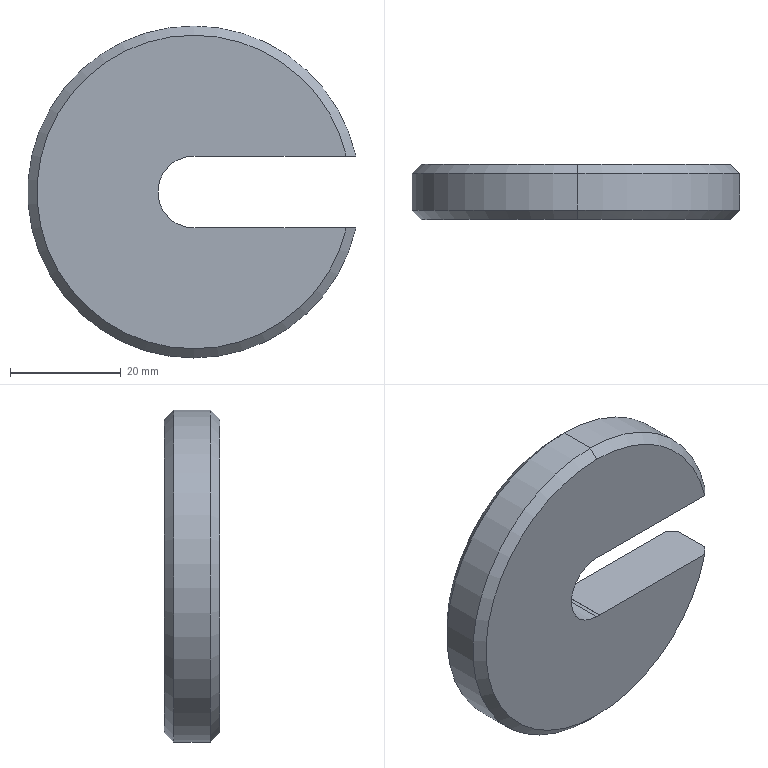Part | SolidWorks | features ICE 2, Chamfer 1, Extrusion 1 | 1 solid | 18 faces | box 59.287 x 10 x 60 mm | volume 23262 mm3 | cone 6 | cylinder 6 | plane 6 | commonest cylinder face diameters 13 x3 60 x3
STEP:
#1=CARTESIAN_POINT('',(0.,10.,28.33));
#2=VERTEX_POINT('',#1);
#3=CARTESIAN_POINT('',(27.574,10.,6.5));
#4=VERTEX_POINT('',#3);
#5=CARTESIAN_POINT('',(0.,10.,0.));
#6=DIRECTION('',(0.,1.,0.));
#7=DIRECTION('',(0.,0.,1.));
#8=AXIS2_PLACEMENT_3D('',#5,#6,#7);
#9=CIRCLE('',#8,28.33);
#10=EDGE_CURVE('',#2,#4,#9,.T.);
#11=ORIENTED_EDGE('',*,*,#10,.F.);
#12=CARTESIAN_POINT('',(0.,8.33,30.));
#13=VERTEX_POINT('',#12);
#14=CARTESIAN_POINT('',(0.,10.,28.33));
#15=DIRECTION('',(0.,-0.7071,0.7071));
#16=VECTOR('',#15,1000.);
#17=LINE('',#14,#16);
#18=EDGE_CURVE('',#2,#13,#17,.T.);
#19=ORIENTED_EDGE('',*,*,#18,.T.);
#20=CARTESIAN_POINT('',(29.287,8.33,6.5));
#21=VERTEX_POINT('',#20);
#22=CARTESIAN_POINT('',(0.,8.33,0.));
#23=DIRECTION('',(0.,-1.,0.));
#24=DIRECTION('',(0.,0.,1.));
#25=AXIS2_PLACEMENT_3D('',#22,#23,#24);
#26=CIRCLE('',#25,30.);
#27=EDGE_CURVE('',#21,#13,#26,.T.);
#28=ORIENTED_EDGE('',*,*,#27,.F.);
#29=CARTESIAN_POINT('',(27.574,10.,6.5));
#30=CARTESIAN_POINT('',(28.146,9.444,6.5));
#31=CARTESIAN_POINT('',(28.717,8.887,6.5));
#32=CARTESIAN_POINT('',(29.287,8.33,6.5));
#33=B_SPLINE_CURVE_WITH_KNOTS('',3,(#29,#30,#31,#32),.UNSPECIFIED.,.F.,.F.,(4,4),(0.,0.002392),.UNSPECIFIED.);
#34=EDGE_CURVE('',#4,#21,#33,.T.);
#35=ORIENTED_EDGE('',*,*,#34,.F.);
#36=EDGE_LOOP('',(#11,#19,#28,#35));
#37=FACE_OUTER_BOUND('',#36,.T.);
#38=CARTESIAN_POINT('',(0.,10.,0.));
#39=DIRECTION('',(0.,-1.,0.));
#40=DIRECTION('',(0.,0.,-1.));
#41=AXIS2_PLACEMENT_3D('',#38,#39,#40);
#42=CONICAL_SURFACE('',#41,28.33,0.7854);
#43=ADVANCED_FACE('',(#37),#42,.T.);
#44=ORIENTED_EDGE('',*,*,#18,.F.);
#45=CARTESIAN_POINT('',(0.,10.,-28.33));
#46=VERTEX_POINT('',#45);
#47=CARTESIAN_POINT('',(0.,10.,0.));
#48=DIRECTION('',(0.,1.,0.));
#49=DIRECTION('',(0.,0.,1.));
#50=AXIS2_PLACEMENT_3D('',#47,#48,#49);
#51=CIRCLE('',#50,28.33);
#52=EDGE_CURVE('',#46,#2,#51,.T.);
#53=ORIENTED_EDGE('',*,*,#52,.F.);
#54=CARTESIAN_POINT('',(0.,8.33,-30.));
#55=VERTEX_POINT('',#54);
#56=CARTESIAN_POINT('',(0.,10.,-28.33));
#57=DIRECTION('',(0.,-0.7071,-0.7071));
#58=VECTOR('',#57,1000.);
#59=LINE('',#56,#58);
#60=EDGE_CURVE('',#46,#55,#59,.T.);
#61=ORIENTED_EDGE('',*,*,#60,.T.);
#62=CARTESIAN_POINT('',(0.,8.33,0.));
#63=DIRECTION('',(0.,-1.,0.));
#64=DIRECTION('',(0.,0.,1.));
#65=AXIS2_PLACEMENT_3D('',#62,#63,#64);
#66=CIRCLE('',#65,30.);
#67=EDGE_CURVE('',#13,#55,#66,.T.);
#68=ORIENTED_EDGE('',*,*,#67,.F.);
#69=EDGE_LOOP('',(#44,#53,#61,#68));
#70=FACE_OUTER_BOUND('',#69,.T.);
#71=CARTESIAN_POINT('',(0.,10.,0.));
#72=DIRECTION('',(0.,-1.,0.));
#73=DIRECTION('',(0.,0.,-1.));
#74=AXIS2_PLACEMENT_3D('',#71,#72,#73);
#75=CONICAL_SURFACE('',#74,28.33,0.7854);
#76=ADVANCED_FACE('',(#70),#75,.T.);
#77=CARTESIAN_POINT('',(0.,0.,-28.33));
#78=VERTEX_POINT('',#77);
#79=CARTESIAN_POINT('',(27.574,0.,-6.5));
#80=VERTEX_POINT('',#79);
#81=CARTESIAN_POINT('',(0.,0.,0.));
#82=DIRECTION('',(0.,-1.,0.));
#83=DIRECTION('',(0.,0.,1.));
#84=AXIS2_PLACEMENT_3D('',#81,#82,#83);
#85=CIRCLE('',#84,28.33);
#86=EDGE_CURVE('',#78,#80,#85,.T.);
#87=ORIENTED_EDGE('',*,*,#86,.F.);
#88=CARTESIAN_POINT('',(0.,1.67,-30.));
#89=VERTEX_POINT('',#88);
#90=CARTESIAN_POINT('',(0.,1.67,-30.));
#91=DIRECTION('',(0.,0.7071,-0.7071));
#92=VECTOR('',#91,1000.);
#93=LINE('',#90,#92);
#94=EDGE_CURVE('',#78,#89,#93,.T.);
#95=ORIENTED_EDGE('',*,*,#94,.T.);
#96=CARTESIAN_POINT('',(29.287,1.67,-6.5));
#97=VERTEX_POINT('',#96);
#98=CARTESIAN_POINT('',(0.,1.67,0.));
#99=DIRECTION('',(0.,1.,0.));
#100=DIRECTION('',(0.,0.,1.));
#101=AXIS2_PLACEMENT_3D('',#98,#99,#100);
#102=CIRCLE('',#101,30.);
#103=EDGE_CURVE('',#97,#89,#102,.T.);
#104=ORIENTED_EDGE('',*,*,#103,.F.);
#105=CARTESIAN_POINT('',(27.574,0.,-6.5));
#106=CARTESIAN_POINT('',(28.146,0.5562,-6.5));
#107=CARTESIAN_POINT('',(28.717,1.113,-6.5));
#108=CARTESIAN_POINT('',(29.287,1.67,-6.5));
#109=B_SPLINE_CURVE_WITH_KNOTS('',3,(#105,#106,#107,#108),.UNSPECIFIED.,.F.,.F.,(4,4),(0.,0.002392),.UNSPECIFIED.);
#110=EDGE_CURVE('',#80,#97,#109,.T.);
#111=ORIENTED_EDGE('',*,*,#110,.F.);
#112=EDGE_LOOP('',(#87,#95,#104,#111));
#113=FACE_OUTER_BOUND('',#112,.T.);
#114=CARTESIAN_POINT('',(0.,1.67,0.));
#115=DIRECTION('',(0.,1.,0.));
#116=DIRECTION('',(0.,0.,1.));
#117=AXIS2_PLACEMENT_3D('',#114,#115,#116);
#118=CONICAL_SURFACE('',#117,30.,0.7854);
#119=ADVANCED_FACE('',(#113),#118,.T.);
#120=ORIENTED_EDGE('',*,*,#94,.F.);
#121=CARTESIAN_POINT('',(0.,0.,28.33));
#122=VERTEX_POINT('',#121);
#123=CARTESIAN_POINT('',(0.,0.,0.));
#124=DIRECTION('',(0.,-1.,0.));
#125=DIRECTION('',(0.,0.,1.));
#126=AXIS2_PLACEMENT_3D('',#123,#124,#125);
#127=CIRCLE('',#126,28.33);
#128=EDGE_CURVE('',#122,#78,#127,.T.);
#129=ORIENTED_EDGE('',*,*,#128,.F.);
#130=CARTESIAN_POINT('',(0.,1.67,30.));
#131=VERTEX_POINT('',#130);
#132=CARTESIAN_POINT('',(0.,1.67,30.));
#133=DIRECTION('',(0.,0.7071,0.7071));
#134=VECTOR('',#133,1000.);
#135=LINE('',#132,#134);
#136=EDGE_CURVE('',#122,#131,#135,.T.);
#137=ORIENTED_EDGE('',*,*,#136,.T.);
#138=CARTESIAN_POINT('',(0.,1.67,0.));
#139=DIRECTION('',(0.,1.,0.));
#140=DIRECTION('',(0.,0.,1.));
#141=AXIS2_PLACEMENT_3D('',#138,#139,#140);
#142=CIRCLE('',#141,30.);
#143=EDGE_CURVE('',#89,#131,#142,.T.);
#144=ORIENTED_EDGE('',*,*,#143,.F.);
#145=EDGE_LOOP('',(#120,#129,#137,#144));
#146=FACE_OUTER_BOUND('',#145,.T.);
#147=CARTESIAN_POINT('',(0.,1.67,0.));
#148=DIRECTION('',(0.,1.,0.));
#149=DIRECTION('',(0.,0.,1.));
#150=AXIS2_PLACEMENT_3D('',#147,#148,#149);
#151=CONICAL_SURFACE('',#150,30.,0.7854);
#152=ADVANCED_FACE('',(#146),#151,.T.);
#153=CARTESIAN_POINT('',(0.,0.,-6.5));
#154=VERTEX_POINT('',#153);
#155=CARTESIAN_POINT('',(0.,0.,6.5));
#156=VERTEX_POINT('',#155);
#157=CARTESIAN_POINT('',(0.,0.,0.));
#158=DIRECTION('',(0.,1.,0.));
#159=DIRECTION('',(0.,0.,1.));
#160=AXIS2_PLACEMENT_3D('',#157,#158,#159);
#161=CIRCLE('',#160,6.5);
#162=EDGE_CURVE('',#154,#156,#161,.T.);
#163=ORIENTED_EDGE('',*,*,#162,.F.);
#164=CARTESIAN_POINT('',(0.,10.,-6.5));
#165=VERTEX_POINT('',#164);
#166=CARTESIAN_POINT('',(0.,-23.,-6.5));
#167=DIRECTION('',(0.,1.,0.));
#168=VECTOR('',#167,1000.);
#169=LINE('',#166,#168);
#170=EDGE_CURVE('',#154,#165,#169,.T.);
#171=ORIENTED_EDGE('',*,*,#170,.T.);
#172=CARTESIAN_POINT('',(0.,10.,6.5));
#173=VERTEX_POINT('',#172);
#174=CARTESIAN_POINT('',(0.,10.,0.));
#175=DIRECTION('',(0.,1.,0.));
#176=DIRECTION('',(0.,0.,1.));
#177=AXIS2_PLACEMENT_3D('',#174,#175,#176);
#178=CIRCLE('',#177,6.5);
#179=EDGE_CURVE('',#165,#173,#178,.T.);
#180=ORIENTED_EDGE('',*,*,#179,.T.);
#181=CARTESIAN_POINT('',(0.,-23.,6.5));
#182=DIRECTION('',(0.,1.,0.));
#183=VECTOR('',#182,1000.);
#184=LINE('',#181,#183);
#185=EDGE_CURVE('',#156,#173,#184,.T.);
#186=ORIENTED_EDGE('',*,*,#185,.F.);
#187=EDGE_LOOP('',(#163,#171,#180,#186));
#188=FACE_OUTER_BOUND('',#187,.T.);
#189=CARTESIAN_POINT('',(0.,-23.,0.));
#190=DIRECTION('',(0.,1.,0.));
#191=DIRECTION('',(0.,0.,1.));
#192=AXIS2_PLACEMENT_3D('',#189,#190,#191);
#193=CYLINDRICAL_SURFACE('',#192,6.5);
#194=ADVANCED_FACE('',(#188),#193,.F.);
#195=CARTESIAN_POINT('',(0.689,0.,6.463));
#196=VERTEX_POINT('',#195);
#197=CARTESIAN_POINT('',(0.,0.,0.));
#198=DIRECTION('',(0.,1.,0.));
#199=DIRECTION('',(0.,0.,1.));
#200=AXIS2_PLACEMENT_3D('',#197,#198,#199);
#201=CIRCLE('',#200,6.5);
#202=EDGE_CURVE('',#156,#196,#201,.T.);
#203=ORIENTED_EDGE('',*,*,#202,.F.);
#204=ORIENTED_EDGE('',*,*,#185,.T.);
#205=CARTESIAN_POINT('',(0.689,10.,6.463));
#206=VERTEX_POINT('',#205);
#207=CARTESIAN_POINT('',(0.,10.,0.));
#208=DIRECTION('',(0.,1.,0.));
#209=DIRECTION('',(0.,0.,1.));
#210=AXIS2_PLACEMENT_3D('',#207,#208,#209);
#211=CIRCLE('',#210,6.5);
#212=EDGE_CURVE('',#173,#206,#211,.T.);
#213=ORIENTED_EDGE('',*,*,#212,.T.);
#214=CARTESIAN_POINT('',(0.689,-23.,6.463));
#215=DIRECTION('',(0.,1.,0.));
#216=VECTOR('',#215,1000.);
#217=LINE('',#214,#216);
#218=EDGE_CURVE('',#196,#206,#217,.T.);
#219=ORIENTED_EDGE('',*,*,#218,.F.);
#220=EDGE_LOOP('',(#203,#204,#213,#219));
#221=FACE_OUTER_BOUND('',#220,.T.);
#222=CARTESIAN_POINT('',(0.,-23.,0.));
#223=DIRECTION('',(0.,1.,0.));
#224=DIRECTION('',(0.,0.,1.));
#225=AXIS2_PLACEMENT_3D('',#222,#223,#224);
#226=CYLINDRICAL_SURFACE('',#225,6.5);
#227=ADVANCED_FACE('',(#221),#226,.F.);
#228=ORIENTED_EDGE('',*,*,#27,.T.);
#229=CARTESIAN_POINT('',(0.,10.,30.));
#230=DIRECTION('',(0.,-1.,0.));
#231=VECTOR('',#230,1000.);
#232=LINE('',#229,#231);
#233=EDGE_CURVE('',#13,#131,#232,.T.);
#234=ORIENTED_EDGE('',*,*,#233,.T.);
#235=CARTESIAN_POINT('',(29.287,1.67,6.5));
#236=VERTEX_POINT('',#235);
#237=CARTESIAN_POINT('',(0.,1.67,0.));
#238=DIRECTION('',(0.,1.,0.));
#239=DIRECTION('',(0.,0.,1.));
#240=AXIS2_PLACEMENT_3D('',#237,#238,#239);
#241=CIRCLE('',#240,30.);
#242=EDGE_CURVE('',#131,#236,#241,.T.);
#243=ORIENTED_EDGE('',*,*,#242,.T.);
#244=CARTESIAN_POINT('',(29.287,10.,6.5));
#245=DIRECTION('',(0.,1.,0.));
#246=VECTOR('',#245,1000.);
#247=LINE('',#244,#246);
#248=EDGE_CURVE('',#236,#21,#247,.T.);
#249=ORIENTED_EDGE('',*,*,#248,.T.);
#250=EDGE_LOOP('',(#228,#234,#243,#249));
#251=FACE_OUTER_BOUND('',#250,.T.);
#252=CARTESIAN_POINT('',(0.,10.,0.));
#253=DIRECTION('',(0.,-1.,0.));
#254=DIRECTION('',(0.,0.,-1.));
#255=AXIS2_PLACEMENT_3D('',#252,#253,#254);
#256=CYLINDRICAL_SURFACE('',#255,30.);
#257=ADVANCED_FACE('',(#251),#256,.T.);
#258=ORIENTED_EDGE('',*,*,#233,.F.);
#259=ORIENTED_EDGE('',*,*,#67,.T.);
#260=CARTESIAN_POINT('',(0.,10.,-30.));
#261=DIRECTION('',(0.,-1.,0.));
#262=VECTOR('',#261,1000.);
#263=LINE('',#260,#262);
#264=EDGE_CURVE('',#55,#89,#263,.T.);
#265=ORIENTED_EDGE('',*,*,#264,.T.);
#266=ORIENTED_EDGE('',*,*,#143,.T.);
#267=EDGE_LOOP('',(#258,#259,#265,#266));
#268=FACE_OUTER_BOUND('',#267,.T.);
#269=CARTESIAN_POINT('',(0.,10.,0.));
#270=DIRECTION('',(0.,-1.,0.));
#271=DIRECTION('',(0.,0.,-1.));
#272=AXIS2_PLACEMENT_3D('',#269,#270,#271);
#273=CYLINDRICAL_SURFACE('',#272,30.);
#274=ADVANCED_FACE('',(#268),#273,.T.);
#275=CARTESIAN_POINT('',(0.689,0.,6.5));
#276=VERTEX_POINT('',#275);
#277=CARTESIAN_POINT('',(0.689,0.,0.));
#278=DIRECTION('',(0.,0.,1.));
#279=VECTOR('',#278,1000.);
#280=LINE('',#277,#279);
#281=EDGE_CURVE('',#196,#276,#280,.T.);
#282=ORIENTED_EDGE('',*,*,#281,.F.);
#283=ORIENTED_EDGE('',*,*,#218,.T.);
#284=CARTESIAN_POINT('',(0.689,10.,6.5));
#285=VERTEX_POINT('',#284);
#286=CARTESIAN_POINT('',(0.689,10.,-6.5));
#287=DIRECTION('',(0.,0.,1.));
#288=VECTOR('',#287,1000.);
#289=LINE('',#286,#288);
#290=EDGE_CURVE('',#206,#285,#289,.T.);
#291=ORIENTED_EDGE('',*,*,#290,.T.);
#292=CARTESIAN_POINT('',(0.689,-23.,6.5));
#293=DIRECTION('',(0.,1.,0.));
#294=VECTOR('',#293,1000.);
#295=LINE('',#292,#294);
#296=EDGE_CURVE('',#276,#285,#295,.T.);
#297=ORIENTED_EDGE('',*,*,#296,.F.);
#298=EDGE_LOOP('',(#282,#283,#291,#297));
#299=FACE_OUTER_BOUND('',#298,.T.);
#300=CARTESIAN_POINT('',(0.689,-23.,-6.5));
#301=DIRECTION('',(-1.,0.,0.));
#302=DIRECTION('',(0.,0.,1.));
#303=AXIS2_PLACEMENT_3D('',#300,#301,#302);
#304=PLANE('',#303);
#305=ADVANCED_FACE('',(#299),#304,.F.);
#306=ORIENTED_EDGE('',*,*,#264,.F.);
#307=CARTESIAN_POINT('',(29.287,8.33,-6.5));
#308=VERTEX_POINT('',#307);
#309=CARTESIAN_POINT('',(0.,8.33,0.));
#310=DIRECTION('',(0.,-1.,0.));
#311=DIRECTION('',(0.,0.,1.));
#312=AXIS2_PLACEMENT_3D('',#309,#310,#311);
#313=CIRCLE('',#312,30.);
#314=EDGE_CURVE('',#55,#308,#313,.T.);
#315=ORIENTED_EDGE('',*,*,#314,.T.);
#316=CARTESIAN_POINT('',(29.287,10.,-6.5));
#317=DIRECTION('',(0.,-1.,0.));
#318=VECTOR('',#317,1000.);
#319=LINE('',#316,#318);
#320=EDGE_CURVE('',#308,#97,#319,.T.);
#321=ORIENTED_EDGE('',*,*,#320,.T.);
#322=ORIENTED_EDGE('',*,*,#103,.T.);
#323=EDGE_LOOP('',(#306,#315,#321,#322));
#324=FACE_OUTER_BOUND('',#323,.T.);
#325=CARTESIAN_POINT('',(0.,10.,0.));
#326=DIRECTION('',(0.,-1.,0.));
#327=DIRECTION('',(0.,0.,-1.));
#328=AXIS2_PLACEMENT_3D('',#325,#326,#327);
#329=CYLINDRICAL_SURFACE('',#328,30.);
#330=ADVANCED_FACE('',(#324),#329,.T.);
#331=CARTESIAN_POINT('',(27.574,10.,-6.5));
#332=VERTEX_POINT('',#331);
#333=CARTESIAN_POINT('',(0.689,10.,-6.5));
#334=VERTEX_POINT('',#333);
#335=CARTESIAN_POINT('',(0.689,10.,-6.5));
#336=DIRECTION('',(-1.,0.,0.));
#337=VECTOR('',#336,1000.);
#338=LINE('',#335,#337);
#339=EDGE_CURVE('',#332,#334,#338,.T.);
#340=ORIENTED_EDGE('',*,*,#339,.F.);
#341=CARTESIAN_POINT('',(0.,10.,0.));
#342=DIRECTION('',(0.,1.,0.));
#343=DIRECTION('',(0.,0.,1.));
#344=AXIS2_PLACEMENT_3D('',#341,#342,#343);
#345=CIRCLE('',#344,28.33);
#346=EDGE_CURVE('',#332,#46,#345,.T.);
#347=ORIENTED_EDGE('',*,*,#346,.T.);
#348=ORIENTED_EDGE('',*,*,#52,.T.);
#349=ORIENTED_EDGE('',*,*,#10,.T.);
#350=CARTESIAN_POINT('',(0.689,10.,6.5));
#351=DIRECTION('',(1.,0.,0.));
#352=VECTOR('',#351,1000.);
#353=LINE('',#350,#352);
#354=EDGE_CURVE('',#285,#4,#353,.T.);
#355=ORIENTED_EDGE('',*,*,#354,.F.);
#356=ORIENTED_EDGE('',*,*,#290,.F.);
#357=ORIENTED_EDGE('',*,*,#212,.F.);
#358=ORIENTED_EDGE('',*,*,#179,.F.);
#359=CARTESIAN_POINT('',(0.689,10.,-6.463));
#360=VERTEX_POINT('',#359);
#361=CARTESIAN_POINT('',(0.,10.,0.));
#362=DIRECTION('',(0.,1.,0.));
#363=DIRECTION('',(0.,0.,1.));
#364=AXIS2_PLACEMENT_3D('',#361,#362,#363);
#365=CIRCLE('',#364,6.5);
#366=EDGE_CURVE('',#360,#165,#365,.T.);
#367=ORIENTED_EDGE('',*,*,#366,.F.);
#368=CARTESIAN_POINT('',(0.689,10.,-6.5));
#369=DIRECTION('',(0.,0.,1.));
#370=VECTOR('',#369,1000.);
#371=LINE('',#368,#370);
#372=EDGE_CURVE('',#334,#360,#371,.T.);
#373=ORIENTED_EDGE('',*,*,#372,.F.);
#374=EDGE_LOOP('',(#340,#347,#348,#349,#355,#356,#357,#358,#367,#373));
#375=FACE_OUTER_BOUND('',#374,.T.);
#376=CARTESIAN_POINT('',(0.,10.,0.));
#377=DIRECTION('',(0.,1.,0.));
#378=DIRECTION('',(0.,0.,1.));
#379=AXIS2_PLACEMENT_3D('',#376,#377,#378);
#380=PLANE('',#379);
#381=ADVANCED_FACE('',(#375),#380,.T.);
#382=CARTESIAN_POINT('',(27.574,0.,6.5));
#383=VERTEX_POINT('',#382);
#384=CARTESIAN_POINT('',(0.,0.,6.5));
#385=DIRECTION('',(1.,0.,0.));
#386=VECTOR('',#385,1000.);
#387=LINE('',#384,#386);
#388=EDGE_CURVE('',#276,#383,#387,.T.);
#389=ORIENTED_EDGE('',*,*,#388,.T.);
#390=CARTESIAN_POINT('',(0.,0.,0.));
#391=DIRECTION('',(0.,-1.,0.));
#392=DIRECTION('',(0.,0.,1.));
#393=AXIS2_PLACEMENT_3D('',#390,#391,#392);
#394=CIRCLE('',#393,28.33);
#395=EDGE_CURVE('',#383,#122,#394,.T.);
#396=ORIENTED_EDGE('',*,*,#395,.T.);
#397=ORIENTED_EDGE('',*,*,#128,.T.);
#398=ORIENTED_EDGE('',*,*,#86,.T.);
#399=CARTESIAN_POINT('',(0.689,0.,-6.5));
#400=VERTEX_POINT('',#399);
#401=CARTESIAN_POINT('',(0.,0.,-6.5));
#402=DIRECTION('',(-1.,0.,0.));
#403=VECTOR('',#402,1000.);
#404=LINE('',#401,#403);
#405=EDGE_CURVE('',#80,#400,#404,.T.);
#406=ORIENTED_EDGE('',*,*,#405,.T.);
#407=CARTESIAN_POINT('',(0.689,0.,-6.463));
#408=VERTEX_POINT('',#407);
#409=CARTESIAN_POINT('',(0.689,0.,0.));
#410=DIRECTION('',(0.,0.,1.));
#411=VECTOR('',#410,1000.);
#412=LINE('',#409,#411);
#413=EDGE_CURVE('',#400,#408,#412,.T.);
#414=ORIENTED_EDGE('',*,*,#413,.T.);
#415=CARTESIAN_POINT('',(0.,0.,0.));
#416=DIRECTION('',(0.,1.,0.));
#417=DIRECTION('',(0.,0.,1.));
#418=AXIS2_PLACEMENT_3D('',#415,#416,#417);
#419=CIRCLE('',#418,6.5);
#420=EDGE_CURVE('',#408,#154,#419,.T.);
#421=ORIENTED_EDGE('',*,*,#420,.T.);
#422=ORIENTED_EDGE('',*,*,#162,.T.);
#423=ORIENTED_EDGE('',*,*,#202,.T.);
#424=ORIENTED_EDGE('',*,*,#281,.T.);
#425=EDGE_LOOP('',(#389,#396,#397,#398,#406,#414,#421,#422,#423,#424));
#426=FACE_OUTER_BOUND('',#425,.T.);
#427=CARTESIAN_POINT('',(0.,0.,0.));
#428=DIRECTION('',(0.,1.,0.));
#429=DIRECTION('',(0.,0.,1.));
#430=AXIS2_PLACEMENT_3D('',#427,#428,#429);
#431=PLANE('',#430);
#432=ADVANCED_FACE('',(#426),#431,.F.);
#433=ORIENTED_EDGE('',*,*,#248,.F.);
#434=CARTESIAN_POINT('',(29.287,1.67,6.5));
#435=CARTESIAN_POINT('',(28.717,1.113,6.5));
#436=CARTESIAN_POINT('',(28.146,0.5562,6.5));
#437=CARTESIAN_POINT('',(27.574,0.,6.5));
#438=B_SPLINE_CURVE_WITH_KNOTS('',3,(#434,#435,#436,#437),.UNSPECIFIED.,.F.,.F.,(4,4),(0.,0.002392),.UNSPECIFIED.);
#439=EDGE_CURVE('',#236,#383,#438,.T.);
#440=ORIENTED_EDGE('',*,*,#439,.T.);
#441=ORIENTED_EDGE('',*,*,#388,.F.);
#442=ORIENTED_EDGE('',*,*,#296,.T.);
#443=ORIENTED_EDGE('',*,*,#354,.T.);
#444=ORIENTED_EDGE('',*,*,#34,.T.);
#445=EDGE_LOOP('',(#433,#440,#441,#442,#443,#444));
#446=FACE_OUTER_BOUND('',#445,.T.);
#447=CARTESIAN_POINT('',(0.689,-23.,6.5));
#448=DIRECTION('',(0.,0.,1.));
#449=DIRECTION('',(1.,0.,0.));
#450=AXIS2_PLACEMENT_3D('',#447,#448,#449);
#451=PLANE('',#450);
#452=ADVANCED_FACE('',(#446),#451,.F.);
#453=ORIENTED_EDGE('',*,*,#372,.T.);
#454=CARTESIAN_POINT('',(0.689,-23.,-6.463));
#455=DIRECTION('',(0.,-1.,0.));
#456=VECTOR('',#455,1000.);
#457=LINE('',#454,#456);
#458=EDGE_CURVE('',#360,#408,#457,.T.);
#459=ORIENTED_EDGE('',*,*,#458,.T.);
#460=ORIENTED_EDGE('',*,*,#413,.F.);
#461=CARTESIAN_POINT('',(0.689,-23.,-6.5));
#462=DIRECTION('',(0.,1.,0.));
#463=VECTOR('',#462,1000.);
#464=LINE('',#461,#463);
#465=EDGE_CURVE('',#400,#334,#464,.T.);
#466=ORIENTED_EDGE('',*,*,#465,.T.);
#467=EDGE_LOOP('',(#453,#459,#460,#466));
#468=FACE_OUTER_BOUND('',#467,.T.);
#469=CARTESIAN_POINT('',(0.689,-23.,-6.5));
#470=DIRECTION('',(-1.,0.,0.));
#471=DIRECTION('',(0.,0.,1.));
#472=AXIS2_PLACEMENT_3D('',#469,#470,#471);
#473=PLANE('',#472);
#474=ADVANCED_FACE('',(#468),#473,.F.);
#475=ORIENTED_EDGE('',*,*,#405,.F.);
#476=ORIENTED_EDGE('',*,*,#110,.T.);
#477=ORIENTED_EDGE('',*,*,#320,.F.);
#478=CARTESIAN_POINT('',(29.287,8.33,-6.5));
#479=CARTESIAN_POINT('',(28.717,8.887,-6.5));
#480=CARTESIAN_POINT('',(28.146,9.444,-6.5));
#481=CARTESIAN_POINT('',(27.574,10.,-6.5));
#482=B_SPLINE_CURVE_WITH_KNOTS('',3,(#478,#479,#480,#481),.UNSPECIFIED.,.F.,.F.,(4,4),(0.,0.002392),.UNSPECIFIED.);
#483=EDGE_CURVE('',#308,#332,#482,.T.);
#484=ORIENTED_EDGE('',*,*,#483,.T.);
#485=ORIENTED_EDGE('',*,*,#339,.T.);
#486=ORIENTED_EDGE('',*,*,#465,.F.);
#487=EDGE_LOOP('',(#475,#476,#477,#484,#485,#486));
#488=FACE_OUTER_BOUND('',#487,.T.);
#489=CARTESIAN_POINT('',(0.689,-23.,-6.5));
#490=DIRECTION('',(0.,0.,-1.));
#491=DIRECTION('',(-1.,0.,0.));
#492=AXIS2_PLACEMENT_3D('',#489,#490,#491);
#493=PLANE('',#492);
#494=ADVANCED_FACE('',(#488),#493,.F.);
#495=ORIENTED_EDGE('',*,*,#170,.F.);
#496=ORIENTED_EDGE('',*,*,#420,.F.);
#497=ORIENTED_EDGE('',*,*,#458,.F.);
#498=ORIENTED_EDGE('',*,*,#366,.T.);
#499=EDGE_LOOP('',(#495,#496,#497,#498));
#500=FACE_OUTER_BOUND('',#499,.T.);
#501=CARTESIAN_POINT('',(0.,-23.,0.));
#502=DIRECTION('',(0.,1.,0.));
#503=DIRECTION('',(0.,0.,1.));
#504=AXIS2_PLACEMENT_3D('',#501,#502,#503);
#505=CYLINDRICAL_SURFACE('',#504,6.5);
#506=ADVANCED_FACE('',(#500),#505,.F.);
#507=ORIENTED_EDGE('',*,*,#136,.F.);
#508=ORIENTED_EDGE('',*,*,#395,.F.);
#509=ORIENTED_EDGE('',*,*,#439,.F.);
#510=ORIENTED_EDGE('',*,*,#242,.F.);
#511=EDGE_LOOP('',(#507,#508,#509,#510));
#512=FACE_OUTER_BOUND('',#511,.T.);
#513=CARTESIAN_POINT('',(0.,1.67,0.));
#514=DIRECTION('',(0.,1.,0.));
#515=DIRECTION('',(0.,0.,1.));
#516=AXIS2_PLACEMENT_3D('',#513,#514,#515);
#517=CONICAL_SURFACE('',#516,30.,0.7854);
#518=ADVANCED_FACE('',(#512),#517,.T.);
#519=ORIENTED_EDGE('',*,*,#60,.F.);
#520=ORIENTED_EDGE('',*,*,#346,.F.);
#521=ORIENTED_EDGE('',*,*,#483,.F.);
#522=ORIENTED_EDGE('',*,*,#314,.F.);
#523=EDGE_LOOP('',(#519,#520,#521,#522));
#524=FACE_OUTER_BOUND('',#523,.T.);
#525=CARTESIAN_POINT('',(0.,10.,0.));
#526=DIRECTION('',(0.,-1.,0.));
#527=DIRECTION('',(0.,0.,-1.));
#528=AXIS2_PLACEMENT_3D('',#525,#526,#527);
#529=CONICAL_SURFACE('',#528,28.33,0.7854);
#530=ADVANCED_FACE('',(#524),#529,.T.);
#531=CLOSED_SHELL('',(#43,#76,#119,#152,#194,#227,#257,#274,#305,#330,#381,#432,#452,#474,#494,#506,#518,#530));
#532=MANIFOLD_SOLID_BREP('',#531);
#533=CARTESIAN_POINT('',(0.,0.,0.));
#534=DIRECTION('',(0.,0.,1.));
#535=DIRECTION('',(1.,0.,0.));
#536=AXIS2_PLACEMENT_3D('',#533,#534,#535);
#537=(LENGTH_UNIT()NAMED_UNIT(*)SI_UNIT(.MILLI.,.METRE.));
#538=UNCERTAINTY_MEASURE_WITH_UNIT(LENGTH_MEASURE(0.00001),#537,'','');
#539=(NAMED_UNIT(*)PLANE_ANGLE_UNIT()SI_UNIT($,.RADIAN.));
#540=(NAMED_UNIT(*)SI_UNIT($,.STERADIAN.)SOLID_ANGLE_UNIT());
#541=(GEOMETRIC_REPRESENTATION_CONTEXT(3)GLOBAL_UNCERTAINTY_ASSIGNED_CONTEXT((#538))GLOBAL_UNIT_ASSIGNED_CONTEXT((#537,#539,#540))REPRESENTATION_CONTEXT('',''));
#542=ADVANCED_BREP_SHAPE_REPRESENTATION('',(#532,#536),#541);